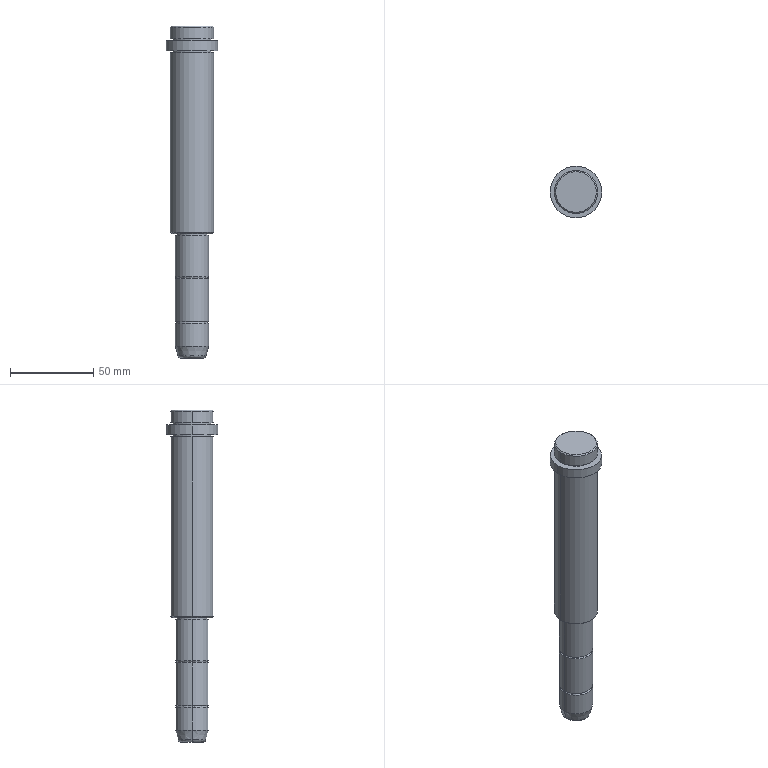Part | STEP file | 38 | 1 solid | 38 faces | box 31 x 31 x 200 mm | volume 90446 mm3 | cylinder 18 | plane 8 | spline 6 | cone 6 | commonest cylinder face diameters 20 x6 23.4 x4 26 x4 18 x2 31 x2